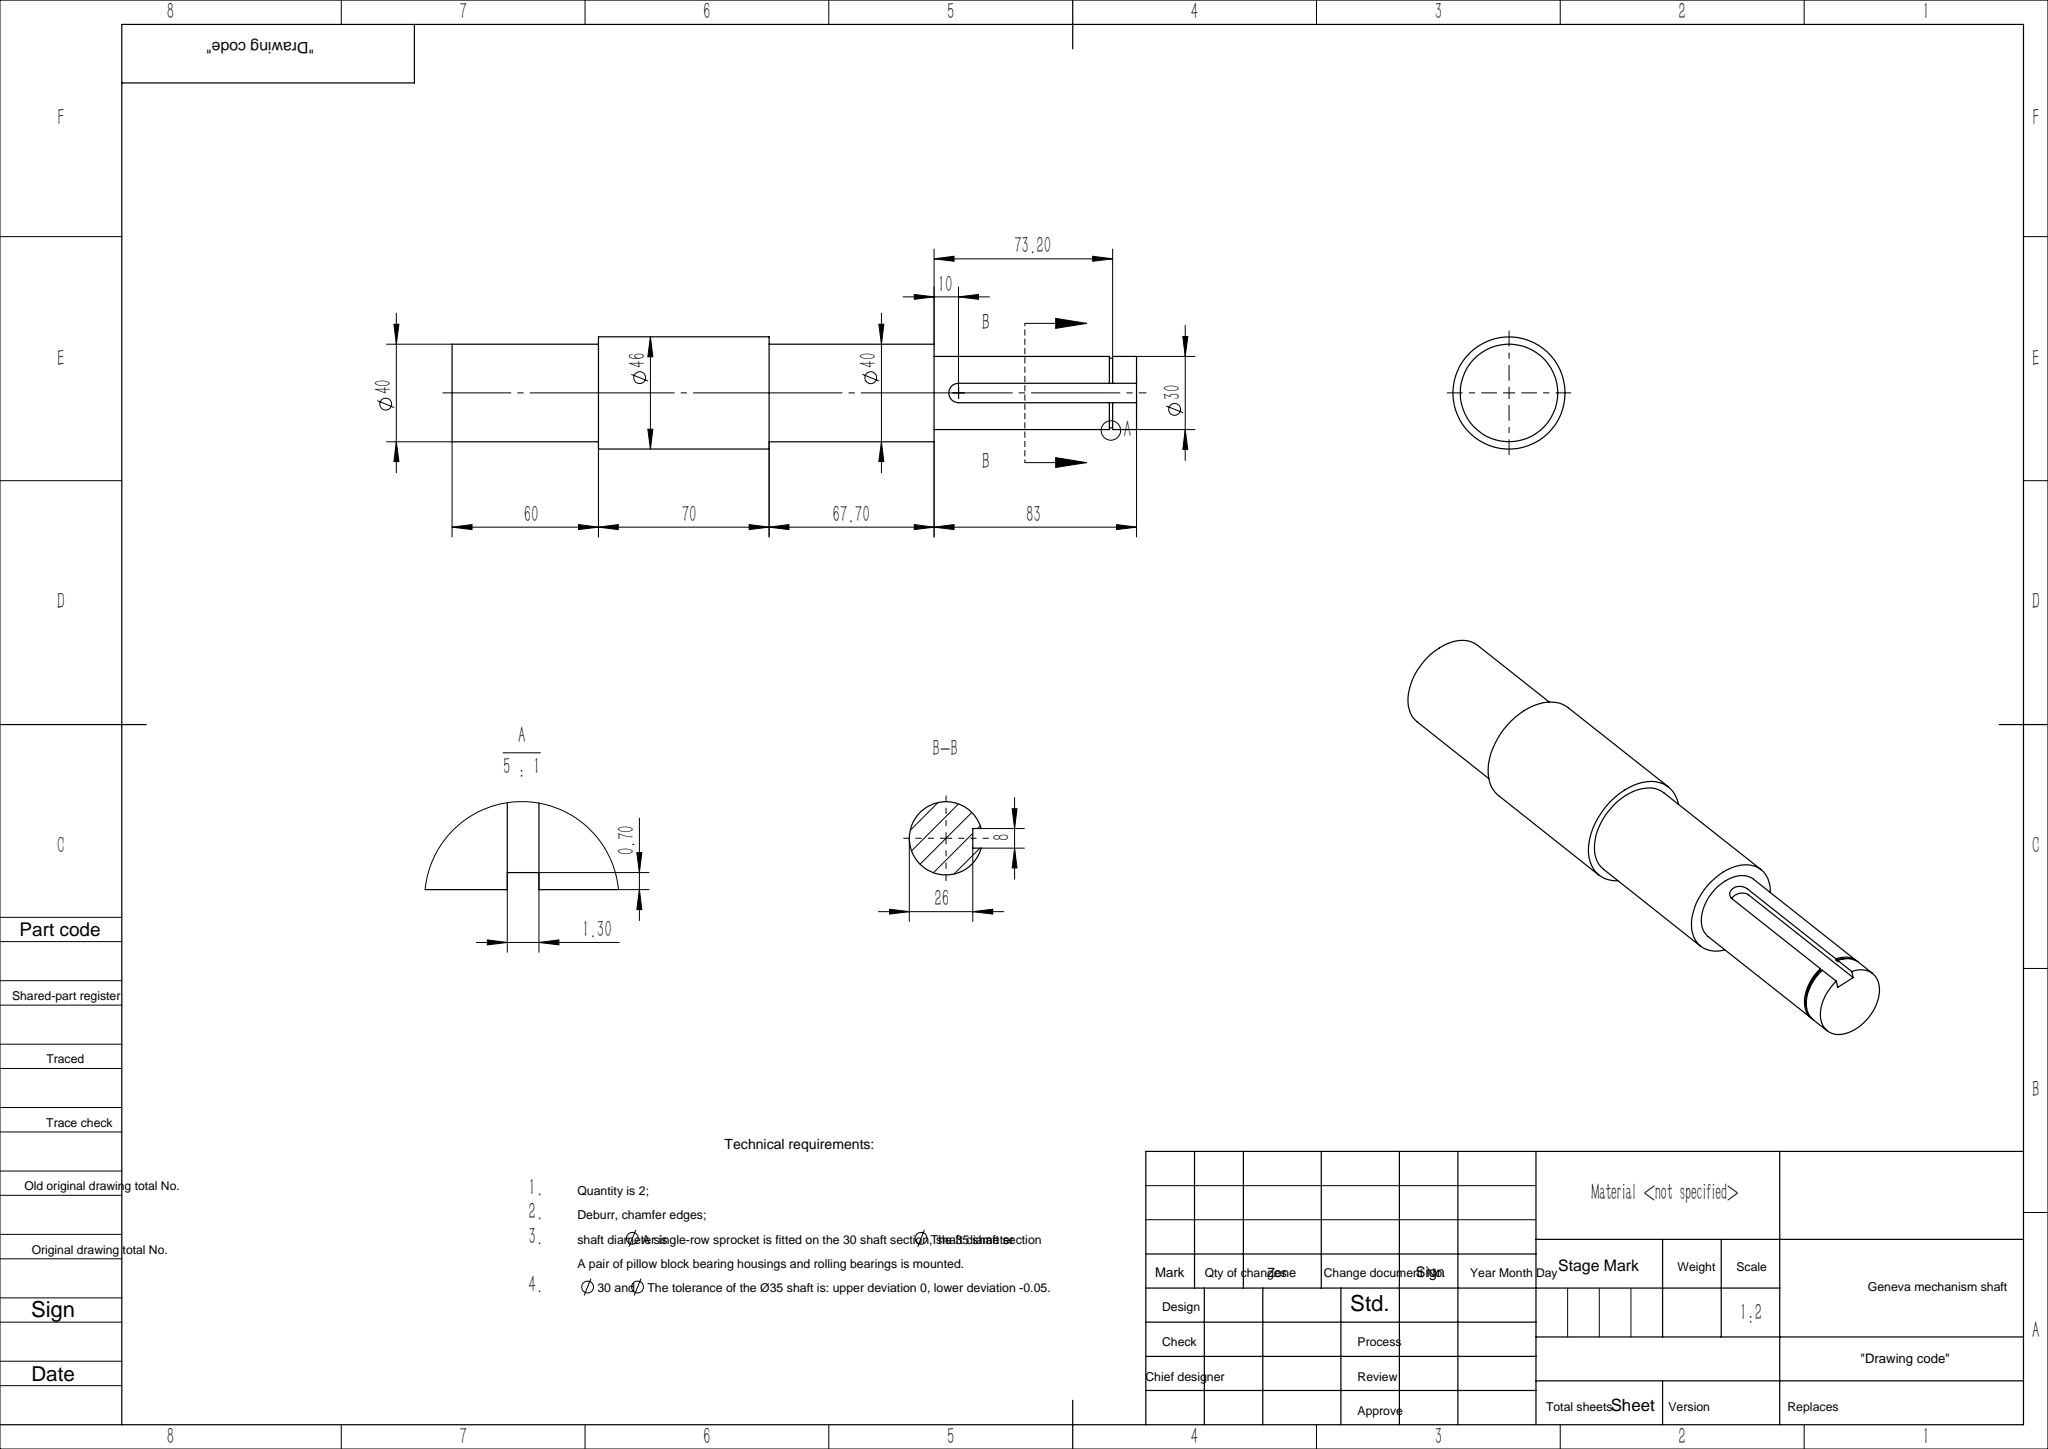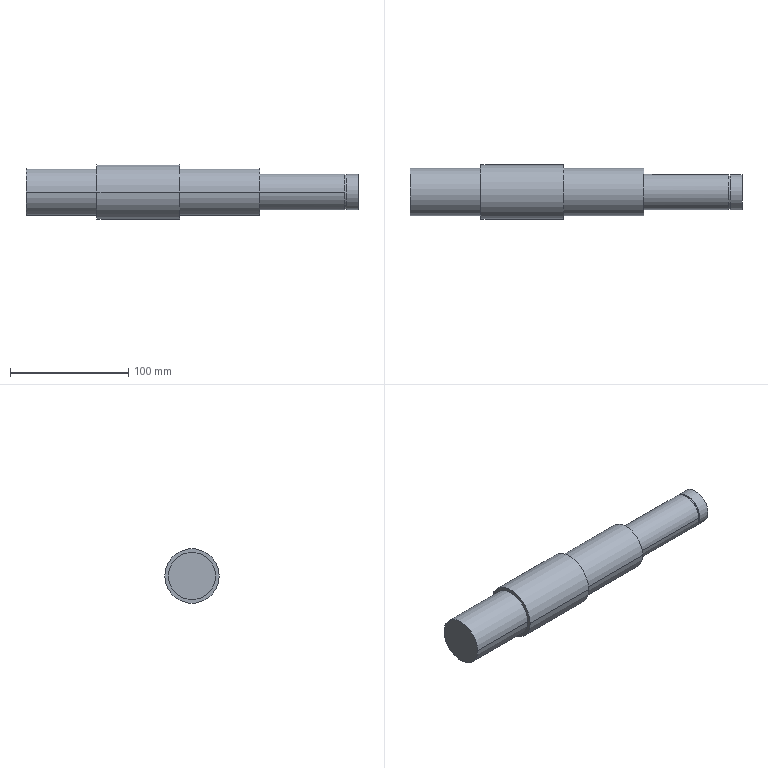Part | SolidWorks | features ICE 2, Revolution 1 | 1 solid | 22 faces | box 280.7 x 46 x 46 mm | volume 333070 mm3 | cylinder 12 | plane 10 | commonest cylinder face diameters 40 x4 30 x3 8 x2 46 x2 28.6 x1
STEP:
#1=CARTESIAN_POINT('',(203.7,11.,0.));
#2=VERTEX_POINT('',#1);
#3=CARTESIAN_POINT('',(207.7,11.,4.));
#4=VERTEX_POINT('',#3);
#5=CARTESIAN_POINT('',(207.7,11.,0.));
#6=DIRECTION('',(0.,1.,0.));
#7=DIRECTION('',(-1.,0.,0.));
#8=AXIS2_PLACEMENT_3D('',#5,#6,#7);
#9=CIRCLE('',#8,4.);
#10=EDGE_CURVE('',#2,#4,#9,.T.);
#11=ORIENTED_EDGE('',*,*,#10,.F.);
#12=CARTESIAN_POINT('',(203.7,15.,0.));
#13=VERTEX_POINT('',#12);
#14=CARTESIAN_POINT('',(203.7,11.,0.));
#15=DIRECTION('',(0.,1.,0.));
#16=VECTOR('',#15,1000.);
#17=LINE('',#14,#16);
#18=EDGE_CURVE('',#2,#13,#17,.T.);
#19=ORIENTED_EDGE('',*,*,#18,.T.);
#20=CARTESIAN_POINT('',(207.7,14.457,4.));
#21=VERTEX_POINT('',#20);
#22=CARTESIAN_POINT('',(203.7,15.,0.));
#23=CARTESIAN_POINT('',(203.7,15.,0.262));
#24=CARTESIAN_POINT('',(203.726,14.993,0.5282));
#25=CARTESIAN_POINT('',(203.829,14.966,1.042));
#26=CARTESIAN_POINT('',(203.905,14.946,1.292));
#27=CARTESIAN_POINT('',(204.208,14.871,2.02));
#28=CARTESIAN_POINT('',(204.502,14.802,2.459));
#29=CARTESIAN_POINT('',(205.057,14.695,3.014));
#30=CARTESIAN_POINT('',(205.257,14.66,3.178));
#31=CARTESIAN_POINT('',(205.689,14.594,3.467));
#32=CARTESIAN_POINT('',(205.923,14.564,3.593));
#33=CARTESIAN_POINT('',(206.405,14.513,3.794));
#34=CARTESIAN_POINT('',(206.654,14.492,3.87));
#35=CARTESIAN_POINT('',(207.169,14.464,3.973));
#36=CARTESIAN_POINT('',(207.435,14.457,4.));
#37=CARTESIAN_POINT('',(207.7,14.457,4.));
#38=B_SPLINE_CURVE_WITH_KNOTS('',3,(#22,#23,#24,#25,#26,#27,#28,#29,#30,#31,#32,#33,#34,#35,#36,#37),.UNSPECIFIED.,.F.,.F.,(4,2,2,2,2,2,2,4),(0.006283,0.007068,0.007852,0.009421,0.01021,0.01099,0.01177,0.01256),.UNSPECIFIED.);
#39=EDGE_CURVE('',#13,#21,#38,.T.);
#40=ORIENTED_EDGE('',*,*,#39,.T.);
#41=CARTESIAN_POINT('',(207.7,11.,4.));
#42=DIRECTION('',(0.,1.,0.));
#43=VECTOR('',#42,1000.);
#44=LINE('',#41,#43);
#45=EDGE_CURVE('',#4,#21,#44,.T.);
#46=ORIENTED_EDGE('',*,*,#45,.F.);
#47=EDGE_LOOP('',(#11,#19,#40,#46));
#48=FACE_OUTER_BOUND('',#47,.T.);
#49=CARTESIAN_POINT('',(207.7,11.,0.));
#50=DIRECTION('',(0.,1.,0.));
#51=DIRECTION('',(-1.,0.,0.));
#52=AXIS2_PLACEMENT_3D('',#49,#50,#51);
#53=CYLINDRICAL_SURFACE('',#52,4.);
#54=ADVANCED_FACE('',(#48),#53,.F.);
#55=CARTESIAN_POINT('',(130.,20.,0.));
#56=VERTEX_POINT('',#55);
#57=CARTESIAN_POINT('',(130.,-20.,0.));
#58=VERTEX_POINT('',#57);
#59=CARTESIAN_POINT('',(130.,0.,0.));
#60=DIRECTION('',(1.,0.,0.));
#61=DIRECTION('',(0.,1.,0.));
#62=AXIS2_PLACEMENT_3D('',#59,#60,#61);
#63=CIRCLE('',#62,20.);
#64=EDGE_CURVE('',#56,#58,#63,.T.);
#65=ORIENTED_EDGE('',*,*,#64,.T.);
#66=CARTESIAN_POINT('',(197.7,-20.,0.));
#67=VERTEX_POINT('',#66);
#68=CARTESIAN_POINT('',(280.7,-20.,0.));
#69=DIRECTION('',(1.,0.,0.));
#70=VECTOR('',#69,1000.);
#71=LINE('',#68,#70);
#72=EDGE_CURVE('',#58,#67,#71,.T.);
#73=ORIENTED_EDGE('',*,*,#72,.T.);
#74=CARTESIAN_POINT('',(197.7,20.,0.));
#75=VERTEX_POINT('',#74);
#76=CARTESIAN_POINT('',(197.7,0.,0.));
#77=DIRECTION('',(1.,0.,0.));
#78=DIRECTION('',(0.,1.,0.));
#79=AXIS2_PLACEMENT_3D('',#76,#77,#78);
#80=CIRCLE('',#79,20.);
#81=EDGE_CURVE('',#75,#67,#80,.T.);
#82=ORIENTED_EDGE('',*,*,#81,.F.);
#83=CARTESIAN_POINT('',(280.7,20.,0.));
#84=DIRECTION('',(1.,0.,0.));
#85=VECTOR('',#84,1000.);
#86=LINE('',#83,#85);
#87=EDGE_CURVE('',#56,#75,#86,.T.);
#88=ORIENTED_EDGE('',*,*,#87,.F.);
#89=EDGE_LOOP('',(#65,#73,#82,#88));
#90=FACE_OUTER_BOUND('',#89,.T.);
#91=CARTESIAN_POINT('',(280.7,0.,0.));
#92=DIRECTION('',(1.,0.,0.));
#93=DIRECTION('',(0.,1.,0.));
#94=AXIS2_PLACEMENT_3D('',#91,#92,#93);
#95=CYLINDRICAL_SURFACE('',#94,20.);
#96=ADVANCED_FACE('',(#90),#95,.T.);
#97=CARTESIAN_POINT('',(60.,23.,0.));
#98=VERTEX_POINT('',#97);
#99=CARTESIAN_POINT('',(60.,-23.,0.));
#100=VERTEX_POINT('',#99);
#101=CARTESIAN_POINT('',(60.,0.,0.));
#102=DIRECTION('',(1.,0.,0.));
#103=DIRECTION('',(0.,1.,0.));
#104=AXIS2_PLACEMENT_3D('',#101,#102,#103);
#105=CIRCLE('',#104,23.);
#106=EDGE_CURVE('',#98,#100,#105,.T.);
#107=ORIENTED_EDGE('',*,*,#106,.T.);
#108=CARTESIAN_POINT('',(130.,-23.,0.));
#109=VERTEX_POINT('',#108);
#110=CARTESIAN_POINT('',(280.7,-23.,0.));
#111=DIRECTION('',(1.,0.,0.));
#112=VECTOR('',#111,1000.);
#113=LINE('',#110,#112);
#114=EDGE_CURVE('',#100,#109,#113,.T.);
#115=ORIENTED_EDGE('',*,*,#114,.T.);
#116=CARTESIAN_POINT('',(130.,23.,0.));
#117=VERTEX_POINT('',#116);
#118=CARTESIAN_POINT('',(130.,0.,0.));
#119=DIRECTION('',(1.,0.,0.));
#120=DIRECTION('',(0.,1.,0.));
#121=AXIS2_PLACEMENT_3D('',#118,#119,#120);
#122=CIRCLE('',#121,23.);
#123=EDGE_CURVE('',#117,#109,#122,.T.);
#124=ORIENTED_EDGE('',*,*,#123,.F.);
#125=CARTESIAN_POINT('',(280.7,23.,0.));
#126=DIRECTION('',(1.,0.,0.));
#127=VECTOR('',#126,1000.);
#128=LINE('',#125,#127);
#129=EDGE_CURVE('',#98,#117,#128,.T.);
#130=ORIENTED_EDGE('',*,*,#129,.F.);
#131=EDGE_LOOP('',(#107,#115,#124,#130));
#132=FACE_OUTER_BOUND('',#131,.T.);
#133=CARTESIAN_POINT('',(280.7,0.,0.));
#134=DIRECTION('',(1.,0.,0.));
#135=DIRECTION('',(0.,1.,0.));
#136=AXIS2_PLACEMENT_3D('',#133,#134,#135);
#137=CYLINDRICAL_SURFACE('',#136,23.);
#138=ADVANCED_FACE('',(#132),#137,.T.);
#139=CARTESIAN_POINT('',(0.,20.,0.));
#140=VERTEX_POINT('',#139);
#141=CARTESIAN_POINT('',(0.,-20.,0.));
#142=VERTEX_POINT('',#141);
#143=CARTESIAN_POINT('',(0.,0.,0.));
#144=DIRECTION('',(1.,0.,0.));
#145=DIRECTION('',(0.,1.,0.));
#146=AXIS2_PLACEMENT_3D('',#143,#144,#145);
#147=CIRCLE('',#146,20.);
#148=EDGE_CURVE('',#140,#142,#147,.T.);
#149=ORIENTED_EDGE('',*,*,#148,.T.);
#150=CARTESIAN_POINT('',(60.,-20.,0.));
#151=VERTEX_POINT('',#150);
#152=CARTESIAN_POINT('',(280.7,-20.,0.));
#153=DIRECTION('',(1.,0.,0.));
#154=VECTOR('',#153,1000.);
#155=LINE('',#152,#154);
#156=EDGE_CURVE('',#142,#151,#155,.T.);
#157=ORIENTED_EDGE('',*,*,#156,.T.);
#158=CARTESIAN_POINT('',(60.,20.,0.));
#159=VERTEX_POINT('',#158);
#160=CARTESIAN_POINT('',(60.,0.,0.));
#161=DIRECTION('',(1.,0.,0.));
#162=DIRECTION('',(0.,1.,0.));
#163=AXIS2_PLACEMENT_3D('',#160,#161,#162);
#164=CIRCLE('',#163,20.);
#165=EDGE_CURVE('',#159,#151,#164,.T.);
#166=ORIENTED_EDGE('',*,*,#165,.F.);
#167=CARTESIAN_POINT('',(280.7,20.,0.));
#168=DIRECTION('',(1.,0.,0.));
#169=VECTOR('',#168,1000.);
#170=LINE('',#167,#169);
#171=EDGE_CURVE('',#140,#159,#170,.T.);
#172=ORIENTED_EDGE('',*,*,#171,.F.);
#173=EDGE_LOOP('',(#149,#157,#166,#172));
#174=FACE_OUTER_BOUND('',#173,.T.);
#175=CARTESIAN_POINT('',(280.7,0.,0.));
#176=DIRECTION('',(1.,0.,0.));
#177=DIRECTION('',(0.,1.,0.));
#178=AXIS2_PLACEMENT_3D('',#175,#176,#177);
#179=CYLINDRICAL_SURFACE('',#178,20.);
#180=ADVANCED_FACE('',(#174),#179,.T.);
#181=CARTESIAN_POINT('',(197.7,15.,0.));
#182=VERTEX_POINT('',#181);
#183=CARTESIAN_POINT('',(197.7,-15.,0.));
#184=VERTEX_POINT('',#183);
#185=CARTESIAN_POINT('',(197.7,0.,0.));
#186=DIRECTION('',(1.,0.,0.));
#187=DIRECTION('',(0.,1.,0.));
#188=AXIS2_PLACEMENT_3D('',#185,#186,#187);
#189=CIRCLE('',#188,15.);
#190=EDGE_CURVE('',#182,#184,#189,.T.);
#191=ORIENTED_EDGE('',*,*,#190,.T.);
#192=CARTESIAN_POINT('',(269.6,-15.,0.));
#193=VERTEX_POINT('',#192);
#194=CARTESIAN_POINT('',(280.7,-15.,0.));
#195=DIRECTION('',(1.,0.,0.));
#196=VECTOR('',#195,1000.);
#197=LINE('',#194,#196);
#198=EDGE_CURVE('',#184,#193,#197,.T.);
#199=ORIENTED_EDGE('',*,*,#198,.T.);
#200=CARTESIAN_POINT('',(269.6,14.457,4.));
#201=VERTEX_POINT('',#200);
#202=CARTESIAN_POINT('',(269.6,0.,0.));
#203=DIRECTION('',(1.,0.,0.));
#204=DIRECTION('',(0.,1.,0.));
#205=AXIS2_PLACEMENT_3D('',#202,#203,#204);
#206=CIRCLE('',#205,15.);
#207=EDGE_CURVE('',#201,#193,#206,.T.);
#208=ORIENTED_EDGE('',*,*,#207,.F.);
#209=CARTESIAN_POINT('',(280.7,14.457,4.));
#210=DIRECTION('',(1.,0.,0.));
#211=VECTOR('',#210,1000.);
#212=LINE('',#209,#211);
#213=EDGE_CURVE('',#21,#201,#212,.T.);
#214=ORIENTED_EDGE('',*,*,#213,.F.);
#215=ORIENTED_EDGE('',*,*,#39,.F.);
#216=CARTESIAN_POINT('',(280.7,15.,0.));
#217=DIRECTION('',(1.,0.,0.));
#218=VECTOR('',#217,1000.);
#219=LINE('',#216,#218);
#220=EDGE_CURVE('',#182,#13,#219,.T.);
#221=ORIENTED_EDGE('',*,*,#220,.F.);
#222=EDGE_LOOP('',(#191,#199,#208,#214,#215,#221));
#223=FACE_OUTER_BOUND('',#222,.T.);
#224=CARTESIAN_POINT('',(280.7,0.,0.));
#225=DIRECTION('',(1.,0.,0.));
#226=DIRECTION('',(0.,1.,0.));
#227=AXIS2_PLACEMENT_3D('',#224,#225,#226);
#228=CYLINDRICAL_SURFACE('',#227,15.);
#229=ADVANCED_FACE('',(#223),#228,.T.);
#230=ORIENTED_EDGE('',*,*,#198,.F.);
#231=CARTESIAN_POINT('',(197.7,0.,0.));
#232=DIRECTION('',(1.,0.,0.));
#233=DIRECTION('',(0.,1.,0.));
#234=AXIS2_PLACEMENT_3D('',#231,#232,#233);
#235=CIRCLE('',#234,15.);
#236=EDGE_CURVE('',#184,#182,#235,.T.);
#237=ORIENTED_EDGE('',*,*,#236,.T.);
#238=ORIENTED_EDGE('',*,*,#220,.T.);
#239=CARTESIAN_POINT('',(207.7,14.457,-4.));
#240=VERTEX_POINT('',#239);
#241=CARTESIAN_POINT('',(207.7,14.457,-4.));
#242=CARTESIAN_POINT('',(207.434,14.457,-4.));
#243=CARTESIAN_POINT('',(207.173,14.464,-3.974));
#244=CARTESIAN_POINT('',(206.66,14.492,-3.871));
#245=CARTESIAN_POINT('',(206.406,14.513,-3.794));
#246=CARTESIAN_POINT('',(205.922,14.564,-3.593));
#247=CARTESIAN_POINT('',(205.692,14.594,-3.47));
#248=CARTESIAN_POINT('',(205.258,14.66,-3.179));
#249=CARTESIAN_POINT('',(205.054,14.696,-3.011));
#250=CARTESIAN_POINT('',(204.687,14.766,-2.644));
#251=CARTESIAN_POINT('',(204.522,14.801,-2.443));
#252=CARTESIAN_POINT('',(204.229,14.867,-2.006));
#253=CARTESIAN_POINT('',(204.106,14.897,-1.775));
#254=CARTESIAN_POINT('',(203.906,14.946,-1.293));
#255=CARTESIAN_POINT('',(203.829,14.966,-1.04));
#256=CARTESIAN_POINT('',(203.726,14.993,-0.5228));
#257=CARTESIAN_POINT('',(203.7,15.,-0.2623));
#258=CARTESIAN_POINT('',(203.7,15.,0.));
#259=B_SPLINE_CURVE_WITH_KNOTS('',3,(#241,#242,#243,#244,#245,#246,#247,#248,#249,#250,#251,#252,#253,#254,#255,#256,#257,#258),.UNSPECIFIED.,.F.,.F.,(4,2,2,2,2,2,2,2,4),(0.,0.0007854,0.001571,0.002356,0.003142,0.003927,0.004712,0.005498,0.006283),.UNSPECIFIED.);
#260=EDGE_CURVE('',#240,#13,#259,.T.);
#261=ORIENTED_EDGE('',*,*,#260,.F.);
#262=CARTESIAN_POINT('',(269.6,14.457,-4.));
#263=VERTEX_POINT('',#262);
#264=CARTESIAN_POINT('',(280.7,14.457,-4.));
#265=DIRECTION('',(-1.,0.,0.));
#266=VECTOR('',#265,1000.);
#267=LINE('',#264,#266);
#268=EDGE_CURVE('',#263,#240,#267,.T.);
#269=ORIENTED_EDGE('',*,*,#268,.F.);
#270=CARTESIAN_POINT('',(269.6,0.,0.));
#271=DIRECTION('',(1.,0.,0.));
#272=DIRECTION('',(0.,1.,0.));
#273=AXIS2_PLACEMENT_3D('',#270,#271,#272);
#274=CIRCLE('',#273,15.);
#275=EDGE_CURVE('',#193,#263,#274,.T.);
#276=ORIENTED_EDGE('',*,*,#275,.F.);
#277=EDGE_LOOP('',(#230,#237,#238,#261,#269,#276));
#278=FACE_OUTER_BOUND('',#277,.T.);
#279=CARTESIAN_POINT('',(280.7,0.,0.));
#280=DIRECTION('',(1.,0.,0.));
#281=DIRECTION('',(0.,1.,0.));
#282=AXIS2_PLACEMENT_3D('',#279,#280,#281);
#283=CYLINDRICAL_SURFACE('',#282,15.);
#284=ADVANCED_FACE('',(#278),#283,.T.);
#285=CARTESIAN_POINT('',(269.6,13.729,-4.));
#286=VERTEX_POINT('',#285);
#287=CARTESIAN_POINT('',(269.6,11.,-4.));
#288=DIRECTION('',(0.,-1.,0.));
#289=VECTOR('',#288,1000.);
#290=LINE('',#287,#289);
#291=EDGE_CURVE('',#263,#286,#290,.T.);
#292=ORIENTED_EDGE('',*,*,#291,.F.);
#293=ORIENTED_EDGE('',*,*,#268,.T.);
#294=CARTESIAN_POINT('',(207.7,11.,-4.));
#295=VERTEX_POINT('',#294);
#296=CARTESIAN_POINT('',(207.7,11.,-4.));
#297=DIRECTION('',(0.,1.,0.));
#298=VECTOR('',#297,1000.);
#299=LINE('',#296,#298);
#300=EDGE_CURVE('',#295,#240,#299,.T.);
#301=ORIENTED_EDGE('',*,*,#300,.F.);
#302=CARTESIAN_POINT('',(280.7,11.,-4.));
#303=VERTEX_POINT('',#302);
#304=CARTESIAN_POINT('',(207.7,11.,-4.));
#305=DIRECTION('',(-1.,0.,0.));
#306=VECTOR('',#305,1000.);
#307=LINE('',#304,#306);
#308=EDGE_CURVE('',#303,#295,#307,.T.);
#309=ORIENTED_EDGE('',*,*,#308,.F.);
#310=CARTESIAN_POINT('',(280.7,14.457,-4.));
#311=VERTEX_POINT('',#310);
#312=CARTESIAN_POINT('',(280.7,15.,-4.));
#313=DIRECTION('',(0.,1.,0.));
#314=VECTOR('',#313,1000.);
#315=LINE('',#312,#314);
#316=EDGE_CURVE('',#303,#311,#315,.T.);
#317=ORIENTED_EDGE('',*,*,#316,.T.);
#318=CARTESIAN_POINT('',(270.9,14.457,-4.));
#319=VERTEX_POINT('',#318);
#320=CARTESIAN_POINT('',(280.7,14.457,-4.));
#321=DIRECTION('',(-1.,0.,0.));
#322=VECTOR('',#321,1000.);
#323=LINE('',#320,#322);
#324=EDGE_CURVE('',#311,#319,#323,.T.);
#325=ORIENTED_EDGE('',*,*,#324,.T.);
#326=CARTESIAN_POINT('',(270.9,13.729,-4.));
#327=VERTEX_POINT('',#326);
#328=CARTESIAN_POINT('',(270.9,11.,-4.));
#329=DIRECTION('',(0.,-1.,0.));
#330=VECTOR('',#329,1000.);
#331=LINE('',#328,#330);
#332=EDGE_CURVE('',#319,#327,#331,.T.);
#333=ORIENTED_EDGE('',*,*,#332,.T.);
#334=CARTESIAN_POINT('',(269.6,13.729,-4.));
#335=DIRECTION('',(1.,0.,0.));
#336=VECTOR('',#335,1000.);
#337=LINE('',#334,#336);
#338=EDGE_CURVE('',#286,#327,#337,.T.);
#339=ORIENTED_EDGE('',*,*,#338,.F.);
#340=EDGE_LOOP('',(#292,#293,#301,#309,#317,#325,#333,#339));
#341=FACE_OUTER_BOUND('',#340,.T.);
#342=CARTESIAN_POINT('',(207.7,11.,-4.));
#343=DIRECTION('',(0.,0.,-1.));
#344=DIRECTION('',(-1.,0.,0.));
#345=AXIS2_PLACEMENT_3D('',#342,#343,#344);
#346=PLANE('',#345);
#347=ADVANCED_FACE('',(#341),#346,.F.);
#348=CARTESIAN_POINT('',(269.6,13.729,4.));
#349=VERTEX_POINT('',#348);
#350=CARTESIAN_POINT('',(269.6,11.,4.));
#351=DIRECTION('',(0.,1.,0.));
#352=VECTOR('',#351,1000.);
#353=LINE('',#350,#352);
#354=EDGE_CURVE('',#349,#201,#353,.T.);
#355=ORIENTED_EDGE('',*,*,#354,.F.);
#356=CARTESIAN_POINT('',(270.9,13.729,4.));
#357=VERTEX_POINT('',#356);
#358=CARTESIAN_POINT('',(269.6,13.729,4.));
#359=DIRECTION('',(-1.,0.,0.));
#360=VECTOR('',#359,1000.);
#361=LINE('',#358,#360);
#362=EDGE_CURVE('',#357,#349,#361,.T.);
#363=ORIENTED_EDGE('',*,*,#362,.F.);
#364=CARTESIAN_POINT('',(270.9,14.457,4.));
#365=VERTEX_POINT('',#364);
#366=CARTESIAN_POINT('',(270.9,11.,4.));
#367=DIRECTION('',(0.,1.,0.));
#368=VECTOR('',#367,1000.);
#369=LINE('',#366,#368);
#370=EDGE_CURVE('',#357,#365,#369,.T.);
#371=ORIENTED_EDGE('',*,*,#370,.T.);
#372=CARTESIAN_POINT('',(280.7,14.457,4.));
#373=VERTEX_POINT('',#372);
#374=CARTESIAN_POINT('',(280.7,14.457,4.));
#375=DIRECTION('',(1.,0.,0.));
#376=VECTOR('',#375,1000.);
#377=LINE('',#374,#376);
#378=EDGE_CURVE('',#365,#373,#377,.T.);
#379=ORIENTED_EDGE('',*,*,#378,.T.);
#380=CARTESIAN_POINT('',(280.7,11.,4.));
#381=VERTEX_POINT('',#380);
#382=CARTESIAN_POINT('',(280.7,15.,4.));
#383=DIRECTION('',(0.,-1.,0.));
#384=VECTOR('',#383,1000.);
#385=LINE('',#382,#384);
#386=EDGE_CURVE('',#373,#381,#385,.T.);
#387=ORIENTED_EDGE('',*,*,#386,.T.);
#388=CARTESIAN_POINT('',(290.7,11.,4.));
#389=DIRECTION('',(1.,0.,0.));
#390=VECTOR('',#389,1000.);
#391=LINE('',#388,#390);
#392=EDGE_CURVE('',#4,#381,#391,.T.);
#393=ORIENTED_EDGE('',*,*,#392,.F.);
#394=ORIENTED_EDGE('',*,*,#45,.T.);
#395=ORIENTED_EDGE('',*,*,#213,.T.);
#396=EDGE_LOOP('',(#355,#363,#371,#379,#387,#393,#394,#395));
#397=FACE_OUTER_BOUND('',#396,.T.);
#398=CARTESIAN_POINT('',(290.7,11.,4.));
#399=DIRECTION('',(0.,0.,1.));
#400=DIRECTION('',(1.,0.,0.));
#401=AXIS2_PLACEMENT_3D('',#398,#399,#400);
#402=PLANE('',#401);
#403=ADVANCED_FACE('',(#397),#402,.F.);
#404=ORIENTED_EDGE('',*,*,#148,.F.);
#405=CARTESIAN_POINT('',(0.,0.,0.));
#406=DIRECTION('',(1.,0.,0.));
#407=DIRECTION('',(0.,1.,0.));
#408=AXIS2_PLACEMENT_3D('',#405,#406,#407);
#409=CIRCLE('',#408,20.);
#410=EDGE_CURVE('',#142,#140,#409,.T.);
#411=ORIENTED_EDGE('',*,*,#410,.F.);
#412=EDGE_LOOP('',(#404,#411));
#413=FACE_OUTER_BOUND('',#412,.T.);
#414=CARTESIAN_POINT('',(0.,0.,0.));
#415=DIRECTION('',(-1.,0.,0.));
#416=DIRECTION('',(0.,-1.,0.));
#417=AXIS2_PLACEMENT_3D('',#414,#415,#416);
#418=PLANE('',#417);
#419=ADVANCED_FACE('',(#413),#418,.T.);
#420=ORIENTED_EDGE('',*,*,#156,.F.);
#421=ORIENTED_EDGE('',*,*,#410,.T.);
#422=ORIENTED_EDGE('',*,*,#171,.T.);
#423=CARTESIAN_POINT('',(60.,0.,0.));
#424=DIRECTION('',(1.,0.,0.));
#425=DIRECTION('',(0.,1.,0.));
#426=AXIS2_PLACEMENT_3D('',#423,#424,#425);
#427=CIRCLE('',#426,20.);
#428=EDGE_CURVE('',#151,#159,#427,.T.);
#429=ORIENTED_EDGE('',*,*,#428,.F.);
#430=EDGE_LOOP('',(#420,#421,#422,#429));
#431=FACE_OUTER_BOUND('',#430,.T.);
#432=CARTESIAN_POINT('',(280.7,0.,0.));
#433=DIRECTION('',(1.,0.,0.));
#434=DIRECTION('',(0.,1.,0.));
#435=AXIS2_PLACEMENT_3D('',#432,#433,#434);
#436=CYLINDRICAL_SURFACE('',#435,20.);
#437=ADVANCED_FACE('',(#431),#436,.T.);
#438=ORIENTED_EDGE('',*,*,#165,.T.);
#439=ORIENTED_EDGE('',*,*,#428,.T.);
#440=EDGE_LOOP('',(#438,#439));
#441=FACE_BOUND('',#440,.T.);
#442=ORIENTED_EDGE('',*,*,#106,.F.);
#443=CARTESIAN_POINT('',(60.,0.,0.));
#444=DIRECTION('',(1.,0.,0.));
#445=DIRECTION('',(0.,1.,0.));
#446=AXIS2_PLACEMENT_3D('',#443,#444,#445);
#447=CIRCLE('',#446,23.);
#448=EDGE_CURVE('',#100,#98,#447,.T.);
#449=ORIENTED_EDGE('',*,*,#448,.F.);
#450=EDGE_LOOP('',(#442,#449));
#451=FACE_OUTER_BOUND('',#450,.T.);
#452=CARTESIAN_POINT('',(60.,20.,0.));
#453=DIRECTION('',(-1.,0.,0.));
#454=DIRECTION('',(0.,-1.,0.));
#455=AXIS2_PLACEMENT_3D('',#452,#453,#454);
#456=PLANE('',#455);
#457=ADVANCED_FACE('',(#441,#451),#456,.T.);
#458=ORIENTED_EDGE('',*,*,#114,.F.);
#459=ORIENTED_EDGE('',*,*,#448,.T.);
#460=ORIENTED_EDGE('',*,*,#129,.T.);
#461=CARTESIAN_POINT('',(130.,0.,0.));
#462=DIRECTION('',(1.,0.,0.));
#463=DIRECTION('',(0.,1.,0.));
#464=AXIS2_PLACEMENT_3D('',#461,#462,#463);
#465=CIRCLE('',#464,23.);
#466=EDGE_CURVE('',#109,#117,#465,.T.);
#467=ORIENTED_EDGE('',*,*,#466,.F.);
#468=EDGE_LOOP('',(#458,#459,#460,#467));
#469=FACE_OUTER_BOUND('',#468,.T.);
#470=CARTESIAN_POINT('',(280.7,0.,0.));
#471=DIRECTION('',(1.,0.,0.));
#472=DIRECTION('',(0.,1.,0.));
#473=AXIS2_PLACEMENT_3D('',#470,#471,#472);
#474=CYLINDRICAL_SURFACE('',#473,23.);
#475=ADVANCED_FACE('',(#469),#474,.T.);
#476=ORIENTED_EDGE('',*,*,#123,.T.);
#477=ORIENTED_EDGE('',*,*,#466,.T.);
#478=EDGE_LOOP('',(#476,#477));
#479=FACE_OUTER_BOUND('',#478,.T.);
#480=ORIENTED_EDGE('',*,*,#64,.F.);
#481=CARTESIAN_POINT('',(130.,0.,0.));
#482=DIRECTION('',(1.,0.,0.));
#483=DIRECTION('',(0.,1.,0.));
#484=AXIS2_PLACEMENT_3D('',#481,#482,#483);
#485=CIRCLE('',#484,20.);
#486=EDGE_CURVE('',#58,#56,#485,.T.);
#487=ORIENTED_EDGE('',*,*,#486,.F.);
#488=EDGE_LOOP('',(#480,#487));
#489=FACE_BOUND('',#488,.T.);
#490=CARTESIAN_POINT('',(130.,23.,0.));
#491=DIRECTION('',(1.,0.,0.));
#492=DIRECTION('',(0.,1.,0.));
#493=AXIS2_PLACEMENT_3D('',#490,#491,#492);
#494=PLANE('',#493);
#495=ADVANCED_FACE('',(#479,#489),#494,.T.);
#496=ORIENTED_EDGE('',*,*,#72,.F.);
#497=ORIENTED_EDGE('',*,*,#486,.T.);
#498=ORIENTED_EDGE('',*,*,#87,.T.);
#499=CARTESIAN_POINT('',(197.7,0.,0.));
#500=DIRECTION('',(1.,0.,0.));
#501=DIRECTION('',(0.,1.,0.));
#502=AXIS2_PLACEMENT_3D('',#499,#500,#501);
#503=CIRCLE('',#502,20.);
#504=EDGE_CURVE('',#67,#75,#503,.T.);
#505=ORIENTED_EDGE('',*,*,#504,.F.);
#506=EDGE_LOOP('',(#496,#497,#498,#505));
#507=FACE_OUTER_BOUND('',#506,.T.);
#508=CARTESIAN_POINT('',(280.7,0.,0.));
#509=DIRECTION('',(1.,0.,0.));
#510=DIRECTION('',(0.,1.,0.));
#511=AXIS2_PLACEMENT_3D('',#508,#509,#510);
#512=CYLINDRICAL_SURFACE('',#511,20.);
#513=ADVANCED_FACE('',(#507),#512,.T.);
#514=ORIENTED_EDGE('',*,*,#81,.T.);
#515=ORIENTED_EDGE('',*,*,#504,.T.);
#516=EDGE_LOOP('',(#514,#515));
#517=FACE_OUTER_BOUND('',#516,.T.);
#518=ORIENTED_EDGE('',*,*,#190,.F.);
#519=ORIENTED_EDGE('',*,*,#236,.F.);
#520=EDGE_LOOP('',(#518,#519));
#521=FACE_BOUND('',#520,.T.);
#522=CARTESIAN_POINT('',(197.7,20.,0.));
#523=DIRECTION('',(1.,0.,0.));
#524=DIRECTION('',(0.,1.,0.));
#525=AXIS2_PLACEMENT_3D('',#522,#523,#524);
#526=PLANE('',#525);
#527=ADVANCED_FACE('',(#517,#521),#526,.T.);
#528=CARTESIAN_POINT('',(270.9,0.,0.));
#529=DIRECTION('',(1.,0.,0.));
#530=DIRECTION('',(0.,1.,0.));
#531=AXIS2_PLACEMENT_3D('',#528,#529,#530);
#532=CIRCLE('',#531,15.);
#533=EDGE_CURVE('',#365,#319,#532,.T.);
#534=ORIENTED_EDGE('',*,*,#533,.T.);
#535=ORIENTED_EDGE('',*,*,#324,.F.);
#536=CARTESIAN_POINT('',(280.7,0.,0.));
#537=DIRECTION('',(1.,0.,0.));
#538=DIRECTION('',(0.,1.,0.));
#539=AXIS2_PLACEMENT_3D('',#536,#537,#538);
#540=CIRCLE('',#539,15.);
#541=EDGE_CURVE('',#373,#311,#540,.T.);
#542=ORIENTED_EDGE('',*,*,#541,.F.);
#543=ORIENTED_EDGE('',*,*,#378,.F.);
#544=EDGE_LOOP('',(#534,#535,#542,#543));
#545=FACE_OUTER_BOUND('',#544,.T.);
#546=CARTESIAN_POINT('',(280.7,0.,0.));
#547=DIRECTION('',(1.,0.,0.));
#548=DIRECTION('',(0.,1.,0.));
#549=AXIS2_PLACEMENT_3D('',#546,#547,#548);
#550=CYLINDRICAL_SURFACE('',#549,15.);
#551=ADVANCED_FACE('',(#545),#550,.T.);
#552=ORIENTED_EDGE('',*,*,#316,.F.);
#553=CARTESIAN_POINT('',(280.7,11.,0.));
#554=DIRECTION('',(0.,0.,1.));
#555=VECTOR('',#554,1000.);
#556=LINE('',#553,#555);
#557=EDGE_CURVE('',#303,#381,#556,.T.);
#558=ORIENTED_EDGE('',*,*,#557,.T.);
#559=ORIENTED_EDGE('',*,*,#386,.F.);
#560=ORIENTED_EDGE('',*,*,#541,.T.);
#561=EDGE_LOOP('',(#552,#558,#559,#560));
#562=FACE_OUTER_BOUND('',#561,.T.);
#563=CARTESIAN_POINT('',(280.7,15.,0.));
#564=DIRECTION('',(1.,0.,0.));
#565=DIRECTION('',(0.,1.,0.));
#566=AXIS2_PLACEMENT_3D('',#563,#564,#565);
#567=PLANE('',#566);
#568=ADVANCED_FACE('',(#562),#567,.T.);
#569=ORIENTED_EDGE('',*,*,#18,.F.);
#570=CARTESIAN_POINT('',(207.7,11.,0.));
#571=DIRECTION('',(0.,1.,0.));
#572=DIRECTION('',(-1.,0.,0.));
#573=AXIS2_PLACEMENT_3D('',#570,#571,#572);
#574=CIRCLE('',#573,4.);
#575=EDGE_CURVE('',#295,#2,#574,.T.);
#576=ORIENTED_EDGE('',*,*,#575,.F.);
#577=ORIENTED_EDGE('',*,*,#300,.T.);
#578=ORIENTED_EDGE('',*,*,#260,.T.);
#579=EDGE_LOOP('',(#569,#576,#577,#578));
#580=FACE_OUTER_BOUND('',#579,.T.);
#581=CARTESIAN_POINT('',(207.7,11.,0.));
#582=DIRECTION('',(0.,1.,0.));
#583=DIRECTION('',(-1.,0.,0.));
#584=AXIS2_PLACEMENT_3D('',#581,#582,#583);
#585=CYLINDRICAL_SURFACE('',#584,4.);
#586=ADVANCED_FACE('',(#580),#585,.F.);
#587=ORIENTED_EDGE('',*,*,#308,.T.);
#588=ORIENTED_EDGE('',*,*,#575,.T.);
#589=ORIENTED_EDGE('',*,*,#10,.T.);
#590=ORIENTED_EDGE('',*,*,#392,.T.);
#591=ORIENTED_EDGE('',*,*,#557,.F.);
#592=EDGE_LOOP('',(#587,#588,#589,#590,#591));
#593=FACE_OUTER_BOUND('',#592,.T.);
#594=CARTESIAN_POINT('',(207.7,11.,0.));
#595=DIRECTION('',(0.,1.,0.));
#596=DIRECTION('',(-1.,0.,0.));
#597=AXIS2_PLACEMENT_3D('',#594,#595,#596);
#598=PLANE('',#597);
#599=ADVANCED_FACE('',(#593),#598,.T.);
#600=ORIENTED_EDGE('',*,*,#291,.T.);
#601=CARTESIAN_POINT('',(269.6,0.,0.));
#602=DIRECTION('',(1.,0.,0.));
#603=DIRECTION('',(0.,1.,0.));
#604=AXIS2_PLACEMENT_3D('',#601,#602,#603);
#605=CIRCLE('',#604,14.3);
#606=EDGE_CURVE('',#349,#286,#605,.T.);
#607=ORIENTED_EDGE('',*,*,#606,.F.);
#608=ORIENTED_EDGE('',*,*,#354,.T.);
#609=ORIENTED_EDGE('',*,*,#207,.T.);
#610=ORIENTED_EDGE('',*,*,#275,.T.);
#611=EDGE_LOOP('',(#600,#607,#608,#609,#610));
#612=FACE_OUTER_BOUND('',#611,.T.);
#613=CARTESIAN_POINT('',(269.6,0.,0.));
#614=DIRECTION('',(1.,0.,0.));
#615=DIRECTION('',(0.,1.,0.));
#616=AXIS2_PLACEMENT_3D('',#613,#614,#615);
#617=PLANE('',#616);
#618=ADVANCED_FACE('',(#612),#617,.T.);
#619=ORIENTED_EDGE('',*,*,#533,.F.);
#620=ORIENTED_EDGE('',*,*,#370,.F.);
#621=CARTESIAN_POINT('',(270.9,0.,0.));
#622=DIRECTION('',(1.,0.,0.));
#623=DIRECTION('',(0.,1.,0.));
#624=AXIS2_PLACEMENT_3D('',#621,#622,#623);
#625=CIRCLE('',#624,14.3);
#626=EDGE_CURVE('',#357,#327,#625,.T.);
#627=ORIENTED_EDGE('',*,*,#626,.T.);
#628=ORIENTED_EDGE('',*,*,#332,.F.);
#629=EDGE_LOOP('',(#619,#620,#627,#628));
#630=FACE_OUTER_BOUND('',#629,.T.);
#631=CARTESIAN_POINT('',(270.9,0.,0.));
#632=DIRECTION('',(1.,0.,0.));
#633=DIRECTION('',(0.,1.,0.));
#634=AXIS2_PLACEMENT_3D('',#631,#632,#633);
#635=PLANE('',#634);
#636=ADVANCED_FACE('',(#630),#635,.F.);
#637=ORIENTED_EDGE('',*,*,#338,.T.);
#638=ORIENTED_EDGE('',*,*,#626,.F.);
#639=ORIENTED_EDGE('',*,*,#362,.T.);
#640=ORIENTED_EDGE('',*,*,#606,.T.);
#641=EDGE_LOOP('',(#637,#638,#639,#640));
#642=FACE_OUTER_BOUND('',#641,.T.);
#643=CARTESIAN_POINT('',(269.6,0.,0.));
#644=DIRECTION('',(1.,0.,0.));
#645=DIRECTION('',(0.,1.,0.));
#646=AXIS2_PLACEMENT_3D('',#643,#644,#645);
#647=CYLINDRICAL_SURFACE('',#646,14.3);
#648=ADVANCED_FACE('',(#642),#647,.T.);
#649=CLOSED_SHELL('',(#54,#96,#138,#180,#229,#284,#347,#403,#419,#437,#457,#475,#495,#513,#527,#551,#568,#586,#599,#618,#636,#648));
#650=MANIFOLD_SOLID_BREP('',#649);
#651=CARTESIAN_POINT('',(0.,0.,0.));
#652=DIRECTION('',(0.,0.,1.));
#653=DIRECTION('',(1.,0.,0.));
#654=AXIS2_PLACEMENT_3D('',#651,#652,#653);
#655=(LENGTH_UNIT()NAMED_UNIT(*)SI_UNIT(.MILLI.,.METRE.));
#656=UNCERTAINTY_MEASURE_WITH_UNIT(LENGTH_MEASURE(0.00001),#655,'','');
#657=(NAMED_UNIT(*)PLANE_ANGLE_UNIT()SI_UNIT($,.RADIAN.));
#658=(NAMED_UNIT(*)SI_UNIT($,.STERADIAN.)SOLID_ANGLE_UNIT());
#659=(GEOMETRIC_REPRESENTATION_CONTEXT(3)GLOBAL_UNCERTAINTY_ASSIGNED_CONTEXT((#656))GLOBAL_UNIT_ASSIGNED_CONTEXT((#655,#657,#658))REPRESENTATION_CONTEXT('',''));
#660=ADVANCED_BREP_SHAPE_REPRESENTATION('',(#650,#654),#659);